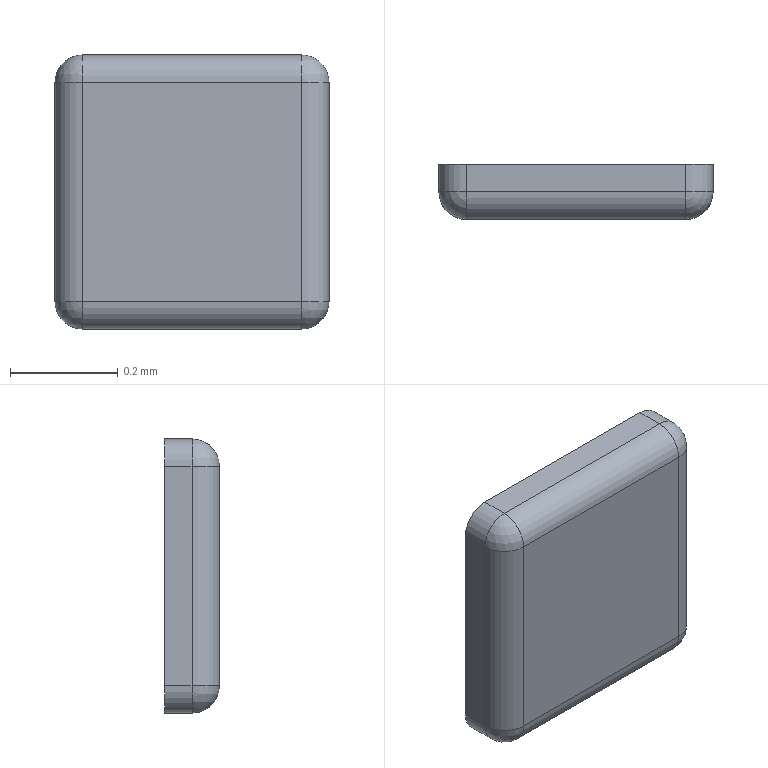Part | STEP file | RJ-USIO-V1_2-220411_2 | 1 solid | 18 faces | box 0.508 x 0.1016 x 0.508 mm | volume 0.02496 mm3 | cylinder 8 | plane 6 | sphere 4 | commonest cylinder face diameters 0.102 x8
STEP:
#1=CARTESIAN_POINT('',(0.,0.,0.));
#2=DIRECTION('',(0.,0.,1.));
#3=DIRECTION('',(1.,0.,0.));
#4=AXIS2_PLACEMENT_3D('',#1,#2,#3);
#5=CARTESIAN_POINT('',(66.597,38.294,0.000000009));
#6=VERTEX_POINT('',#5);
#7=CARTESIAN_POINT('',(67.003,38.294,-0.000000009));
#8=VERTEX_POINT('',#7);
#9=CARTESIAN_POINT('',(66.597,38.294,0.000000009));
#10=DIRECTION('',(1.,0.000000044,-0.000000044));
#11=VECTOR('',#10,1.);
#12=LINE('',#9,#11);
#13=CARTESIAN_POINT('',(67.054,38.294,0.508));
#14=DIRECTION('',(-0.000000044,1.,0.));
#15=DIRECTION('',(1.,0.000000044,-0.000000044));
#16=AXIS2_PLACEMENT_3D('',#13,#14,#15);
#17=PLANE('',#16);
#18=CARTESIAN_POINT('',(-0.4572,0.508));
#19=DIRECTION('',(1.,0.));
#20=VECTOR('',#19,1.);
#21=LINE('',#18,#20);
#22=(GEOMETRIC_REPRESENTATION_CONTEXT(2)PARAMETRIC_REPRESENTATION_CONTEXT()REPRESENTATION_CONTEXT('',''));
#23=DEFINITIONAL_REPRESENTATION('',(#21),#22);
#24=PCURVE('',#17,#23);
#25=CARTESIAN_POINT('',(66.546,38.192,0.000000011));
#26=DIRECTION('',(0.000000044,0.,1.));
#27=DIRECTION('',(-1.,-0.000000044,0.000000044));
#28=AXIS2_PLACEMENT_3D('',#25,#26,#27);
#29=PLANE('',#28);
#30=CARTESIAN_POINT('',(-0.0508,-0.1016));
#31=DIRECTION('',(-1.,0.));
#32=VECTOR('',#31,1.);
#33=LINE('',#30,#32);
#34=(GEOMETRIC_REPRESENTATION_CONTEXT(2)PARAMETRIC_REPRESENTATION_CONTEXT()REPRESENTATION_CONTEXT('',''));
#35=DEFINITIONAL_REPRESENTATION('',(#33),#34);
#36=PCURVE('',#29,#35);
#37=SURFACE_CURVE('',#12,(#24,#36),.PCURVE_S1.);
#38=EDGE_CURVE('',#6,#8,#37,.T.);
#39=ORIENTED_EDGE('',*,*,#38,.T.);
#40=CARTESIAN_POINT('',(67.054,38.294,0.0508));
#41=VERTEX_POINT('',#40);
#42=CARTESIAN_POINT('',(67.003,38.294,0.0508));
#43=DIRECTION('',(-0.000000044,1.,0.));
#44=DIRECTION('',(1.,0.000000044,-0.000000044));
#45=AXIS2_PLACEMENT_3D('',#42,#43,#44);
#46=CIRCLE('',#45,0.0508);
#47=CARTESIAN_POINT('',(-0.0508,0.4572));
#48=DIRECTION('',(1.,0.));
#49=AXIS2_PLACEMENT_2D('',#47,#48);
#50=CIRCLE('',#49,0.0508);
#51=(GEOMETRIC_REPRESENTATION_CONTEXT(2)PARAMETRIC_REPRESENTATION_CONTEXT()REPRESENTATION_CONTEXT('',''));
#52=DEFINITIONAL_REPRESENTATION('',(#50),#51);
#53=PCURVE('',#17,#52);
#54=CARTESIAN_POINT('',(67.003,38.192,0.0508));
#55=DIRECTION('',(-0.000000044,1.,0.));
#56=DIRECTION('',(1.,0.000000044,-0.000000044));
#57=AXIS2_PLACEMENT_3D('',#54,#55,#56);
#58=CYLINDRICAL_SURFACE('',#57,0.0508);
#59=CARTESIAN_POINT('',(0.,0.1016));
#60=DIRECTION('',(1.,0.));
#61=VECTOR('',#60,1.);
#62=LINE('',#59,#61);
#63=(GEOMETRIC_REPRESENTATION_CONTEXT(2)PARAMETRIC_REPRESENTATION_CONTEXT()REPRESENTATION_CONTEXT('',''));
#64=DEFINITIONAL_REPRESENTATION('',(#62),#63);
#65=PCURVE('',#58,#64);
#66=SURFACE_CURVE('',#46,(#53,#65),.PCURVE_S1.);
#67=EDGE_CURVE('',#41,#8,#66,.T.);
#68=ORIENTED_EDGE('',*,*,#67,.F.);
#69=CARTESIAN_POINT('',(67.054,38.294,0.4572));
#70=VERTEX_POINT('',#69);
#71=CARTESIAN_POINT('',(67.054,38.294,0.0508));
#72=DIRECTION('',(0.000000044,0.,1.));
#73=VECTOR('',#72,1.);
#74=LINE('',#71,#73);
#75=CARTESIAN_POINT('',(0.,0.4572));
#76=DIRECTION('',(0.,-1.));
#77=VECTOR('',#76,1.);
#78=LINE('',#75,#77);
#79=(GEOMETRIC_REPRESENTATION_CONTEXT(2)PARAMETRIC_REPRESENTATION_CONTEXT()REPRESENTATION_CONTEXT('',''));
#80=DEFINITIONAL_REPRESENTATION('',(#78),#79);
#81=PCURVE('',#17,#80);
#82=CARTESIAN_POINT('',(67.054,38.192,-0.000000011));
#83=DIRECTION('',(-1.,-0.000000044,0.000000044));
#84=DIRECTION('',(-0.000000044,1.,0.));
#85=AXIS2_PLACEMENT_3D('',#82,#83,#84);
#86=PLANE('',#85);
#87=CARTESIAN_POINT('',(0.1016,-0.0508));
#88=DIRECTION('',(0.,-1.));
#89=VECTOR('',#88,1.);
#90=LINE('',#87,#89);
#91=(GEOMETRIC_REPRESENTATION_CONTEXT(2)PARAMETRIC_REPRESENTATION_CONTEXT()REPRESENTATION_CONTEXT('',''));
#92=DEFINITIONAL_REPRESENTATION('',(#90),#91);
#93=PCURVE('',#86,#92);
#94=SURFACE_CURVE('',#74,(#81,#93),.PCURVE_S1.);
#95=EDGE_CURVE('',#41,#70,#94,.T.);
#96=ORIENTED_EDGE('',*,*,#95,.T.);
#97=CARTESIAN_POINT('',(67.003,38.294,0.508));
#98=VERTEX_POINT('',#97);
#99=CARTESIAN_POINT('',(67.003,38.294,0.4572));
#100=DIRECTION('',(-0.000000044,1.,0.));
#101=DIRECTION('',(0.000000044,0.,1.));
#102=AXIS2_PLACEMENT_3D('',#99,#100,#101);
#103=CIRCLE('',#102,0.0508);
#104=CARTESIAN_POINT('',(-0.0508,0.0508));
#105=DIRECTION('',(0.,-1.));
#106=AXIS2_PLACEMENT_2D('',#104,#105);
#107=CIRCLE('',#106,0.0508);
#108=(GEOMETRIC_REPRESENTATION_CONTEXT(2)PARAMETRIC_REPRESENTATION_CONTEXT()REPRESENTATION_CONTEXT('',''));
#109=DEFINITIONAL_REPRESENTATION('',(#107),#108);
#110=PCURVE('',#17,#109);
#111=CARTESIAN_POINT('',(67.003,38.192,0.4572));
#112=DIRECTION('',(-0.000000044,1.,0.));
#113=DIRECTION('',(1.,0.000000044,-0.000000044));
#114=AXIS2_PLACEMENT_3D('',#111,#112,#113);
#115=CYLINDRICAL_SURFACE('',#114,0.0508);
#116=CARTESIAN_POINT('',(4.712,0.1016));
#117=DIRECTION('',(1.,0.));
#118=VECTOR('',#117,1.);
#119=LINE('',#116,#118);
#120=(GEOMETRIC_REPRESENTATION_CONTEXT(2)PARAMETRIC_REPRESENTATION_CONTEXT()REPRESENTATION_CONTEXT('',''));
#121=DEFINITIONAL_REPRESENTATION('',(#119),#120);
#122=PCURVE('',#115,#121);
#123=SURFACE_CURVE('',#103,(#110,#122),.PCURVE_S1.);
#124=EDGE_CURVE('',#98,#70,#123,.T.);
#125=ORIENTED_EDGE('',*,*,#124,.F.);
#126=CARTESIAN_POINT('',(66.597,38.294,0.508));
#127=VERTEX_POINT('',#126);
#128=CARTESIAN_POINT('',(67.003,38.294,0.508));
#129=DIRECTION('',(-1.,-0.000000044,0.000000044));
#130=VECTOR('',#129,1.);
#131=LINE('',#128,#130);
#132=CARTESIAN_POINT('',(-0.0508,0.));
#133=DIRECTION('',(-1.,0.));
#134=VECTOR('',#133,1.);
#135=LINE('',#132,#134);
#136=(GEOMETRIC_REPRESENTATION_CONTEXT(2)PARAMETRIC_REPRESENTATION_CONTEXT()REPRESENTATION_CONTEXT('',''));
#137=DEFINITIONAL_REPRESENTATION('',(#135),#136);
#138=PCURVE('',#17,#137);
#139=CARTESIAN_POINT('',(66.546,38.192,0.508));
#140=DIRECTION('',(-0.000000044,0.,-1.));
#141=DIRECTION('',(1.,0.000000044,-0.000000044));
#142=AXIS2_PLACEMENT_3D('',#139,#140,#141);
#143=PLANE('',#142);
#144=CARTESIAN_POINT('',(0.4572,-0.1016));
#145=DIRECTION('',(-1.,0.));
#146=VECTOR('',#145,1.);
#147=LINE('',#144,#146);
#148=(GEOMETRIC_REPRESENTATION_CONTEXT(2)PARAMETRIC_REPRESENTATION_CONTEXT()REPRESENTATION_CONTEXT('',''));
#149=DEFINITIONAL_REPRESENTATION('',(#147),#148);
#150=PCURVE('',#143,#149);
#151=SURFACE_CURVE('',#131,(#138,#150),.PCURVE_S1.);
#152=EDGE_CURVE('',#98,#127,#151,.T.);
#153=ORIENTED_EDGE('',*,*,#152,.T.);
#154=CARTESIAN_POINT('',(66.546,38.294,0.4572));
#155=VERTEX_POINT('',#154);
#156=CARTESIAN_POINT('',(66.597,38.294,0.4572));
#157=DIRECTION('',(-0.000000044,1.,0.));
#158=DIRECTION('',(-1.,-0.000000044,0.000000044));
#159=AXIS2_PLACEMENT_3D('',#156,#157,#158);
#160=CIRCLE('',#159,0.0508);
#161=CARTESIAN_POINT('',(-0.4572,0.0508));
#162=DIRECTION('',(-1.,0.));
#163=AXIS2_PLACEMENT_2D('',#161,#162);
#164=CIRCLE('',#163,0.0508);
#165=(GEOMETRIC_REPRESENTATION_CONTEXT(2)PARAMETRIC_REPRESENTATION_CONTEXT()REPRESENTATION_CONTEXT('',''));
#166=DEFINITIONAL_REPRESENTATION('',(#164),#165);
#167=PCURVE('',#17,#166);
#168=CARTESIAN_POINT('',(66.597,38.192,0.4572));
#169=DIRECTION('',(-0.000000044,1.,0.));
#170=DIRECTION('',(1.,0.000000044,-0.000000044));
#171=AXIS2_PLACEMENT_3D('',#168,#169,#170);
#172=CYLINDRICAL_SURFACE('',#171,0.0508);
#173=CARTESIAN_POINT('',(3.142,0.1016));
#174=DIRECTION('',(1.,0.));
#175=VECTOR('',#174,1.);
#176=LINE('',#173,#175);
#177=(GEOMETRIC_REPRESENTATION_CONTEXT(2)PARAMETRIC_REPRESENTATION_CONTEXT()REPRESENTATION_CONTEXT('',''));
#178=DEFINITIONAL_REPRESENTATION('',(#176),#177);
#179=PCURVE('',#172,#178);
#180=SURFACE_CURVE('',#160,(#167,#179),.PCURVE_S1.);
#181=EDGE_CURVE('',#155,#127,#180,.T.);
#182=ORIENTED_EDGE('',*,*,#181,.F.);
#183=CARTESIAN_POINT('',(66.546,38.294,0.0508));
#184=VERTEX_POINT('',#183);
#185=CARTESIAN_POINT('',(66.546,38.294,0.4572));
#186=DIRECTION('',(-0.000000044,0.,-1.));
#187=VECTOR('',#186,1.);
#188=LINE('',#185,#187);
#189=CARTESIAN_POINT('',(-0.508,0.0508));
#190=DIRECTION('',(0.,1.));
#191=VECTOR('',#190,1.);
#192=LINE('',#189,#191);
#193=(GEOMETRIC_REPRESENTATION_CONTEXT(2)PARAMETRIC_REPRESENTATION_CONTEXT()REPRESENTATION_CONTEXT('',''));
#194=DEFINITIONAL_REPRESENTATION('',(#192),#193);
#195=PCURVE('',#17,#194);
#196=CARTESIAN_POINT('',(66.546,38.192,0.000000011));
#197=DIRECTION('',(1.,0.000000044,-0.000000044));
#198=DIRECTION('',(0.000000044,-1.,0.));
#199=AXIS2_PLACEMENT_3D('',#196,#197,#198);
#200=PLANE('',#199);
#201=CARTESIAN_POINT('',(-0.1016,-0.4572));
#202=DIRECTION('',(0.,1.));
#203=VECTOR('',#202,1.);
#204=LINE('',#201,#203);
#205=(GEOMETRIC_REPRESENTATION_CONTEXT(2)PARAMETRIC_REPRESENTATION_CONTEXT()REPRESENTATION_CONTEXT('',''));
#206=DEFINITIONAL_REPRESENTATION('',(#204),#205);
#207=PCURVE('',#200,#206);
#208=SURFACE_CURVE('',#188,(#195,#207),.PCURVE_S1.);
#209=EDGE_CURVE('',#155,#184,#208,.T.);
#210=ORIENTED_EDGE('',*,*,#209,.T.);
#211=CARTESIAN_POINT('',(66.597,38.294,0.0508));
#212=DIRECTION('',(-0.000000044,1.,0.));
#213=DIRECTION('',(-0.000000044,0.,-1.));
#214=AXIS2_PLACEMENT_3D('',#211,#212,#213);
#215=CIRCLE('',#214,0.0508);
#216=CARTESIAN_POINT('',(-0.4572,0.4572));
#217=DIRECTION('',(0.,1.));
#218=AXIS2_PLACEMENT_2D('',#216,#217);
#219=CIRCLE('',#218,0.0508);
#220=(GEOMETRIC_REPRESENTATION_CONTEXT(2)PARAMETRIC_REPRESENTATION_CONTEXT()REPRESENTATION_CONTEXT('',''));
#221=DEFINITIONAL_REPRESENTATION('',(#219),#220);
#222=PCURVE('',#17,#221);
#223=CARTESIAN_POINT('',(66.597,38.192,0.0508));
#224=DIRECTION('',(-0.000000044,1.,0.));
#225=DIRECTION('',(1.,0.000000044,-0.000000044));
#226=AXIS2_PLACEMENT_3D('',#223,#224,#225);
#227=CYLINDRICAL_SURFACE('',#226,0.0508);
#228=CARTESIAN_POINT('',(1.571,0.1016));
#229=DIRECTION('',(1.,0.));
#230=VECTOR('',#229,1.);
#231=LINE('',#228,#230);
#232=(GEOMETRIC_REPRESENTATION_CONTEXT(2)PARAMETRIC_REPRESENTATION_CONTEXT()REPRESENTATION_CONTEXT('',''));
#233=DEFINITIONAL_REPRESENTATION('',(#231),#232);
#234=PCURVE('',#227,#233);
#235=SURFACE_CURVE('',#215,(#222,#234),.PCURVE_S1.);
#236=EDGE_CURVE('',#6,#184,#235,.T.);
#237=ORIENTED_EDGE('',*,*,#236,.F.);
#238=EDGE_LOOP('',(#39,#68,#96,#125,#153,#182,#210,#237));
#239=FACE_BOUND('',#238,.F.);
#240=ADVANCED_FACE('',(#239),#17,.T.);
#241=CARTESIAN_POINT('',(66.597,38.243,0.000000009));
#242=VERTEX_POINT('',#241);
#243=CARTESIAN_POINT('',(67.003,38.243,-0.000000009));
#244=VERTEX_POINT('',#243);
#245=CARTESIAN_POINT('',(66.597,38.243,0.000000009));
#246=DIRECTION('',(1.,0.000000044,-0.000000044));
#247=VECTOR('',#246,1.);
#248=LINE('',#245,#247);
#249=CARTESIAN_POINT('',(-0.0508,-0.0508));
#250=DIRECTION('',(-1.,0.));
#251=VECTOR('',#250,1.);
#252=LINE('',#249,#251);
#253=(GEOMETRIC_REPRESENTATION_CONTEXT(2)PARAMETRIC_REPRESENTATION_CONTEXT()REPRESENTATION_CONTEXT('',''));
#254=DEFINITIONAL_REPRESENTATION('',(#252),#253);
#255=PCURVE('',#29,#254);
#256=CARTESIAN_POINT('',(67.054,38.243,0.0508));
#257=DIRECTION('',(1.,0.000000044,-0.000000044));
#258=DIRECTION('',(0.000000044,-1.,0.));
#259=AXIS2_PLACEMENT_3D('',#256,#257,#258);
#260=CYLINDRICAL_SURFACE('',#259,0.0508);
#261=CARTESIAN_POINT('',(1.571,-0.4572));
#262=DIRECTION('',(0.,1.));
#263=VECTOR('',#262,1.);
#264=LINE('',#261,#263);
#265=(GEOMETRIC_REPRESENTATION_CONTEXT(2)PARAMETRIC_REPRESENTATION_CONTEXT()REPRESENTATION_CONTEXT('',''));
#266=DEFINITIONAL_REPRESENTATION('',(#264),#265);
#267=PCURVE('',#260,#266);
#268=SURFACE_CURVE('',#248,(#255,#267),.PCURVE_S1.);
#269=EDGE_CURVE('',#242,#244,#268,.T.);
#270=ORIENTED_EDGE('',*,*,#269,.T.);
#271=CARTESIAN_POINT('',(67.003,38.243,-0.000000009));
#272=DIRECTION('',(-0.000000044,1.,0.));
#273=VECTOR('',#272,1.);
#274=LINE('',#271,#273);
#275=CARTESIAN_POINT('',(-0.4572,-0.0508));
#276=DIRECTION('',(0.,-1.));
#277=VECTOR('',#276,1.);
#278=LINE('',#275,#277);
#279=(GEOMETRIC_REPRESENTATION_CONTEXT(2)PARAMETRIC_REPRESENTATION_CONTEXT()REPRESENTATION_CONTEXT('',''));
#280=DEFINITIONAL_REPRESENTATION('',(#278),#279);
#281=PCURVE('',#29,#280);
#282=CARTESIAN_POINT('',(1.571,0.0508));
#283=DIRECTION('',(0.,1.));
#284=VECTOR('',#283,1.);
#285=LINE('',#282,#284);
#286=(GEOMETRIC_REPRESENTATION_CONTEXT(2)PARAMETRIC_REPRESENTATION_CONTEXT()REPRESENTATION_CONTEXT('',''));
#287=DEFINITIONAL_REPRESENTATION('',(#285),#286);
#288=PCURVE('',#58,#287);
#289=SURFACE_CURVE('',#274,(#281,#288),.PCURVE_S1.);
#290=EDGE_CURVE('',#244,#8,#289,.T.);
#291=ORIENTED_EDGE('',*,*,#290,.T.);
#292=ORIENTED_EDGE('',*,*,#38,.F.);
#293=CARTESIAN_POINT('',(66.597,38.294,0.000000009));
#294=DIRECTION('',(0.000000044,-1.,0.));
#295=VECTOR('',#294,1.);
#296=LINE('',#293,#295);
#297=CARTESIAN_POINT('',(-0.0508,-0.1016));
#298=DIRECTION('',(0.,1.));
#299=VECTOR('',#298,1.);
#300=LINE('',#297,#299);
#301=(GEOMETRIC_REPRESENTATION_CONTEXT(2)PARAMETRIC_REPRESENTATION_CONTEXT()REPRESENTATION_CONTEXT('',''));
#302=DEFINITIONAL_REPRESENTATION('',(#300),#301);
#303=PCURVE('',#29,#302);
#304=CARTESIAN_POINT('',(1.571,0.1016));
#305=DIRECTION('',(0.,-1.));
#306=VECTOR('',#305,1.);
#307=LINE('',#304,#306);
#308=(GEOMETRIC_REPRESENTATION_CONTEXT(2)PARAMETRIC_REPRESENTATION_CONTEXT()REPRESENTATION_CONTEXT('',''));
#309=DEFINITIONAL_REPRESENTATION('',(#307),#308);
#310=PCURVE('',#227,#309);
#311=SURFACE_CURVE('',#296,(#303,#310),.PCURVE_S1.);
#312=EDGE_CURVE('',#6,#242,#311,.T.);
#313=ORIENTED_EDGE('',*,*,#312,.T.);
#314=EDGE_LOOP('',(#270,#291,#292,#313));
#315=FACE_BOUND('',#314,.F.);
#316=ADVANCED_FACE('',(#315),#29,.F.);
#317=CARTESIAN_POINT('',(67.003,38.192,0.0508));
#318=VERTEX_POINT('',#317);
#319=CARTESIAN_POINT('',(66.597,38.192,0.0508));
#320=VERTEX_POINT('',#319);
#321=CARTESIAN_POINT('',(67.003,38.192,0.0508));
#322=DIRECTION('',(-1.,-0.000000044,0.000000044));
#323=VECTOR('',#322,1.);
#324=LINE('',#321,#323);
#325=CARTESIAN_POINT('',(0.,-0.0508));
#326=DIRECTION('',(0.,-1.));
#327=VECTOR('',#326,1.);
#328=LINE('',#325,#327);
#329=(GEOMETRIC_REPRESENTATION_CONTEXT(2)PARAMETRIC_REPRESENTATION_CONTEXT()REPRESENTATION_CONTEXT('',''));
#330=DEFINITIONAL_REPRESENTATION('',(#328),#329);
#331=PCURVE('',#260,#330);
#332=CARTESIAN_POINT('',(67.054,38.192,0.508));
#333=DIRECTION('',(-0.000000044,1.,0.));
#334=DIRECTION('',(1.,0.000000044,-0.000000044));
#335=AXIS2_PLACEMENT_3D('',#332,#333,#334);
#336=PLANE('',#335);
#337=CARTESIAN_POINT('',(-0.0508,0.4572));
#338=DIRECTION('',(-1.,0.));
#339=VECTOR('',#338,1.);
#340=LINE('',#337,#339);
#341=(GEOMETRIC_REPRESENTATION_CONTEXT(2)PARAMETRIC_REPRESENTATION_CONTEXT()REPRESENTATION_CONTEXT('',''));
#342=DEFINITIONAL_REPRESENTATION('',(#340),#341);
#343=PCURVE('',#336,#342);
#344=SURFACE_CURVE('',#324,(#331,#343),.PCURVE_S1.);
#345=EDGE_CURVE('',#318,#320,#344,.T.);
#346=ORIENTED_EDGE('',*,*,#345,.T.);
#347=CARTESIAN_POINT('',(66.597,38.243,0.0508));
#348=DIRECTION('',(-1.,-0.000000044,0.000000044));
#349=DIRECTION('',(-0.000000044,0.,-1.));
#350=AXIS2_PLACEMENT_3D('',#347,#348,#349);
#351=CIRCLE('',#350,0.0508);
#352=CARTESIAN_POINT('',(1.571,-0.4572));
#353=DIRECTION('',(-1.,0.));
#354=VECTOR('',#353,1.);
#355=LINE('',#352,#354);
#356=(GEOMETRIC_REPRESENTATION_CONTEXT(2)PARAMETRIC_REPRESENTATION_CONTEXT()REPRESENTATION_CONTEXT('',''));
#357=DEFINITIONAL_REPRESENTATION('',(#355),#356);
#358=PCURVE('',#260,#357);
#359=CARTESIAN_POINT('',(66.597,38.243,0.0508));
#360=DIRECTION('',(0.000000044,0.,1.));
#361=DIRECTION('',(1.,0.000000044,-0.000000044));
#362=AXIS2_PLACEMENT_3D('',#359,#360,#361);
#363=SPHERICAL_SURFACE('',#362,0.0508);
#364=CARTESIAN_POINT('',(4.712,-1.571));
#365=DIRECTION('',(0.,1.));
#366=VECTOR('',#365,1.);
#367=LINE('',#364,#366);
#368=(GEOMETRIC_REPRESENTATION_CONTEXT(2)PARAMETRIC_REPRESENTATION_CONTEXT()REPRESENTATION_CONTEXT('',''));
#369=DEFINITIONAL_REPRESENTATION('',(#367),#368);
#370=PCURVE('',#363,#369);
#371=SURFACE_CURVE('',#351,(#358,#370),.PCURVE_S1.);
#372=EDGE_CURVE('',#242,#320,#371,.T.);
#373=ORIENTED_EDGE('',*,*,#372,.F.);
#374=ORIENTED_EDGE('',*,*,#269,.T.);
#375=CARTESIAN_POINT('',(67.003,38.243,0.0508));
#376=DIRECTION('',(1.,0.000000044,-0.000000044));
#377=DIRECTION('',(0.000000044,-1.,0.));
#378=AXIS2_PLACEMENT_3D('',#375,#376,#377);
#379=CIRCLE('',#378,0.0508);
#380=CARTESIAN_POINT('',(0.,-0.0508));
#381=DIRECTION('',(1.,0.));
#382=VECTOR('',#381,1.);
#383=LINE('',#380,#382);
#384=(GEOMETRIC_REPRESENTATION_CONTEXT(2)PARAMETRIC_REPRESENTATION_CONTEXT()REPRESENTATION_CONTEXT('',''));
#385=DEFINITIONAL_REPRESENTATION('',(#383),#384);
#386=PCURVE('',#260,#385);
#387=CARTESIAN_POINT('',(67.003,38.243,0.0508));
#388=DIRECTION('',(0.000000044,0.,1.));
#389=DIRECTION('',(1.,0.000000044,-0.000000044));
#390=AXIS2_PLACEMENT_3D('',#387,#388,#389);
#391=SPHERICAL_SURFACE('',#390,0.0508);
#392=CARTESIAN_POINT('',(4.712,0.));
#393=CARTESIAN_POINT('',(4.712,-0.0238));
#394=CARTESIAN_POINT('',(4.712,-0.0714));
#395=CARTESIAN_POINT('',(4.712,-0.1428));
#396=CARTESIAN_POINT('',(4.712,-0.2142));
#397=CARTESIAN_POINT('',(4.712,-0.2856));
#398=CARTESIAN_POINT('',(4.712,-0.357));
#399=CARTESIAN_POINT('',(4.712,-0.4284));
#400=CARTESIAN_POINT('',(4.712,-0.4998));
#401=CARTESIAN_POINT('',(4.712,-0.5712));
#402=CARTESIAN_POINT('',(4.712,-0.6426));
#403=CARTESIAN_POINT('',(4.712,-0.714));
#404=CARTESIAN_POINT('',(4.712,-0.7854));
#405=CARTESIAN_POINT('',(4.712,-0.8568));
#406=CARTESIAN_POINT('',(4.712,-0.9282));
#407=CARTESIAN_POINT('',(4.712,-0.9996));
#408=CARTESIAN_POINT('',(4.712,-1.071));
#409=CARTESIAN_POINT('',(4.712,-1.142));
#410=CARTESIAN_POINT('',(4.712,-1.214));
#411=CARTESIAN_POINT('',(4.712,-1.285));
#412=CARTESIAN_POINT('',(4.712,-1.357));
#413=CARTESIAN_POINT('',(4.712,-1.428));
#414=CARTESIAN_POINT('',(4.712,-1.499));
#415=CARTESIAN_POINT('',(4.712,-1.547));
#416=CARTESIAN_POINT('',(4.712,-1.571));
#417=B_SPLINE_CURVE_WITH_KNOTS('',3,(#392,#393,#394,#395,#396,#397,#398,#399,#400,#401,#402,#403,#404,#405,#406,#407,#408,#409,#410,#411,#412,#413,#414,#415,#416),.UNSPECIFIED.,.F.,.F.,(4,1,1,1,1,1,1,1,1,1,1,1,1,1,1,1,1,1,1,1,1,1,4),(0.,0.0714,0.1428,0.2142,0.2856,0.357,0.4284,0.4998,0.5712,0.6426,0.714,0.7854,0.8568,0.9282,0.9996,1.071,1.142,1.214,1.285,1.357,1.428,1.499,1.571),.QUASI_UNIFORM_KNOTS.);
#418=(GEOMETRIC_REPRESENTATION_CONTEXT(2)PARAMETRIC_REPRESENTATION_CONTEXT()REPRESENTATION_CONTEXT('',''));
#419=DEFINITIONAL_REPRESENTATION('',(#417),#418);
#420=PCURVE('',#391,#419);
#421=SURFACE_CURVE('',#379,(#386,#420),.PCURVE_S1.);
#422=EDGE_CURVE('',#318,#244,#421,.T.);
#423=ORIENTED_EDGE('',*,*,#422,.F.);
#424=EDGE_LOOP('',(#346,#373,#374,#423));
#425=FACE_BOUND('',#424,.T.);
#426=ADVANCED_FACE('',(#425),#260,.T.);
#427=CARTESIAN_POINT('',(67.054,38.243,0.0508));
#428=VERTEX_POINT('',#427);
#429=CARTESIAN_POINT('',(67.003,38.243,0.0508));
#430=DIRECTION('',(-0.000000044,0.,-1.));
#431=DIRECTION('',(1.,0.000000044,-0.000000044));
#432=AXIS2_PLACEMENT_3D('',#429,#430,#431);
#433=CIRCLE('',#432,0.0508);
#434=CARTESIAN_POINT('',(6.283,0.));
#435=DIRECTION('',(-1.,0.));
#436=VECTOR('',#435,1.);
#437=LINE('',#434,#436);
#438=(GEOMETRIC_REPRESENTATION_CONTEXT(2)PARAMETRIC_REPRESENTATION_CONTEXT()REPRESENTATION_CONTEXT('',''));
#439=DEFINITIONAL_REPRESENTATION('',(#437),#438);
#440=PCURVE('',#391,#439);
#441=CARTESIAN_POINT('',(67.003,38.243,0.508));
#442=DIRECTION('',(0.000000044,0.,1.));
#443=DIRECTION('',(-1.,-0.000000044,0.000000044));
#444=AXIS2_PLACEMENT_3D('',#441,#442,#443);
#445=CYLINDRICAL_SURFACE('',#444,0.0508);
#446=CARTESIAN_POINT('',(3.142,-0.4572));
#447=DIRECTION('',(-1.,0.));
#448=VECTOR('',#447,1.);
#449=LINE('',#446,#448);
#450=(GEOMETRIC_REPRESENTATION_CONTEXT(2)PARAMETRIC_REPRESENTATION_CONTEXT()REPRESENTATION_CONTEXT('',''));
#451=DEFINITIONAL_REPRESENTATION('',(#449),#450);
#452=PCURVE('',#445,#451);
#453=SURFACE_CURVE('',#433,(#440,#452),.PCURVE_S1.);
#454=EDGE_CURVE('',#428,#318,#453,.T.);
#455=ORIENTED_EDGE('',*,*,#454,.T.);
#456=ORIENTED_EDGE('',*,*,#422,.T.);
#457=CARTESIAN_POINT('',(67.003,38.243,0.0508));
#458=DIRECTION('',(0.000000044,-1.,0.));
#459=DIRECTION('',(-0.000000044,0.,-1.));
#460=AXIS2_PLACEMENT_3D('',#457,#458,#459);
#461=CIRCLE('',#460,0.0508);
#462=CARTESIAN_POINT('',(6.283,-1.571));
#463=DIRECTION('',(0.,1.));
#464=VECTOR('',#463,1.);
#465=LINE('',#462,#464);
#466=(GEOMETRIC_REPRESENTATION_CONTEXT(2)PARAMETRIC_REPRESENTATION_CONTEXT()REPRESENTATION_CONTEXT('',''));
#467=DEFINITIONAL_REPRESENTATION('',(#465),#466);
#468=PCURVE('',#391,#467);
#469=CARTESIAN_POINT('',(1.571,0.0508));
#470=DIRECTION('',(-1.,0.));
#471=VECTOR('',#470,1.);
#472=LINE('',#469,#471);
#473=(GEOMETRIC_REPRESENTATION_CONTEXT(2)PARAMETRIC_REPRESENTATION_CONTEXT()REPRESENTATION_CONTEXT('',''));
#474=DEFINITIONAL_REPRESENTATION('',(#472),#473);
#475=PCURVE('',#58,#474);
#476=SURFACE_CURVE('',#461,(#468,#475),.PCURVE_S1.);
#477=EDGE_CURVE('',#244,#428,#476,.T.);
#478=ORIENTED_EDGE('',*,*,#477,.T.);
#479=EDGE_LOOP('',(#455,#456,#478));
#480=FACE_BOUND('',#479,.T.);
#481=ADVANCED_FACE('',(#480),#391,.T.);
#482=ORIENTED_EDGE('',*,*,#67,.F.);
#483=CARTESIAN_POINT('',(67.054,38.294,0.0508));
#484=DIRECTION('',(0.000000044,-1.,0.));
#485=VECTOR('',#484,1.);
#486=LINE('',#483,#485);
#487=CARTESIAN_POINT('',(0.,0.1016));
#488=DIRECTION('',(0.,-1.));
#489=VECTOR('',#488,1.);
#490=LINE('',#487,#489);
#491=(GEOMETRIC_REPRESENTATION_CONTEXT(2)PARAMETRIC_REPRESENTATION_CONTEXT()REPRESENTATION_CONTEXT('',''));
#492=DEFINITIONAL_REPRESENTATION('',(#490),#491);
#493=PCURVE('',#58,#492);
#494=CARTESIAN_POINT('',(0.1016,-0.0508));
#495=DIRECTION('',(-1.,0.));
#496=VECTOR('',#495,1.);
#497=LINE('',#494,#496);
#498=(GEOMETRIC_REPRESENTATION_CONTEXT(2)PARAMETRIC_REPRESENTATION_CONTEXT()REPRESENTATION_CONTEXT('',''));
#499=DEFINITIONAL_REPRESENTATION('',(#497),#498);
#500=PCURVE('',#86,#499);
#501=SURFACE_CURVE('',#486,(#493,#500),.PCURVE_S1.);
#502=EDGE_CURVE('',#41,#428,#501,.T.);
#503=ORIENTED_EDGE('',*,*,#502,.T.);
#504=ORIENTED_EDGE('',*,*,#477,.F.);
#505=ORIENTED_EDGE('',*,*,#290,.T.);
#506=EDGE_LOOP('',(#482,#503,#504,#505));
#507=FACE_BOUND('',#506,.T.);
#508=ADVANCED_FACE('',(#507),#58,.T.);
#509=CARTESIAN_POINT('',(67.054,38.243,0.4572));
#510=VERTEX_POINT('',#509);
#511=CARTESIAN_POINT('',(67.054,38.243,0.0508));
#512=DIRECTION('',(0.000000044,0.,1.));
#513=VECTOR('',#512,1.);
#514=LINE('',#511,#513);
#515=CARTESIAN_POINT('',(0.0508,-0.0508));
#516=DIRECTION('',(0.,-1.));
#517=VECTOR('',#516,1.);
#518=LINE('',#515,#517);
#519=(GEOMETRIC_REPRESENTATION_CONTEXT(2)PARAMETRIC_REPRESENTATION_CONTEXT()REPRESENTATION_CONTEXT('',''));
#520=DEFINITIONAL_REPRESENTATION('',(#518),#519);
#521=PCURVE('',#86,#520);
#522=CARTESIAN_POINT('',(3.142,-0.4572));
#523=DIRECTION('',(0.,1.));
#524=VECTOR('',#523,1.);
#525=LINE('',#522,#524);
#526=(GEOMETRIC_REPRESENTATION_CONTEXT(2)PARAMETRIC_REPRESENTATION_CONTEXT()REPRESENTATION_CONTEXT('',''));
#527=DEFINITIONAL_REPRESENTATION('',(#525),#526);
#528=PCURVE('',#445,#527);
#529=SURFACE_CURVE('',#514,(#521,#528),.PCURVE_S1.);
#530=EDGE_CURVE('',#428,#510,#529,.T.);
#531=ORIENTED_EDGE('',*,*,#530,.T.);
#532=CARTESIAN_POINT('',(67.054,38.243,0.4572));
#533=DIRECTION('',(-0.000000044,1.,0.));
#534=VECTOR('',#533,1.);
#535=LINE('',#532,#534);
#536=CARTESIAN_POINT('',(0.0508,-0.4572));
#537=DIRECTION('',(1.,0.));
#538=VECTOR('',#537,1.);
#539=LINE('',#536,#538);
#540=(GEOMETRIC_REPRESENTATION_CONTEXT(2)PARAMETRIC_REPRESENTATION_CONTEXT()REPRESENTATION_CONTEXT('',''));
#541=DEFINITIONAL_REPRESENTATION('',(#539),#540);
#542=PCURVE('',#86,#541);
#543=CARTESIAN_POINT('',(6.283,0.0508));
#544=DIRECTION('',(0.,1.));
#545=VECTOR('',#544,1.);
#546=LINE('',#543,#545);
#547=(GEOMETRIC_REPRESENTATION_CONTEXT(2)PARAMETRIC_REPRESENTATION_CONTEXT()REPRESENTATION_CONTEXT('',''));
#548=DEFINITIONAL_REPRESENTATION('',(#546),#547);
#549=PCURVE('',#115,#548);
#550=SURFACE_CURVE('',#535,(#542,#549),.PCURVE_S1.);
#551=EDGE_CURVE('',#510,#70,#550,.T.);
#552=ORIENTED_EDGE('',*,*,#551,.T.);
#553=ORIENTED_EDGE('',*,*,#95,.F.);
#554=ORIENTED_EDGE('',*,*,#502,.T.);
#555=EDGE_LOOP('',(#531,#552,#553,#554));
#556=FACE_BOUND('',#555,.F.);
#557=ADVANCED_FACE('',(#556),#86,.F.);
#558=CARTESIAN_POINT('',(67.003,38.192,0.4572));
#559=VERTEX_POINT('',#558);
#560=CARTESIAN_POINT('',(67.003,38.192,0.4572));
#561=DIRECTION('',(-0.000000044,0.,-1.));
#562=VECTOR('',#561,1.);
#563=LINE('',#560,#562);
#564=CARTESIAN_POINT('',(1.571,-0.0508));
#565=DIRECTION('',(0.,-1.));
#566=VECTOR('',#565,1.);
#567=LINE('',#564,#566);
#568=(GEOMETRIC_REPRESENTATION_CONTEXT(2)PARAMETRIC_REPRESENTATION_CONTEXT()REPRESENTATION_CONTEXT('',''));
#569=DEFINITIONAL_REPRESENTATION('',(#567),#568);
#570=PCURVE('',#445,#569);
#571=CARTESIAN_POINT('',(-0.0508,0.0508));
#572=DIRECTION('',(0.,1.));
#573=VECTOR('',#572,1.);
#574=LINE('',#571,#573);
#575=(GEOMETRIC_REPRESENTATION_CONTEXT(2)PARAMETRIC_REPRESENTATION_CONTEXT()REPRESENTATION_CONTEXT('',''));
#576=DEFINITIONAL_REPRESENTATION('',(#574),#575);
#577=PCURVE('',#336,#576);
#578=SURFACE_CURVE('',#563,(#570,#577),.PCURVE_S1.);
#579=EDGE_CURVE('',#559,#318,#578,.T.);
#580=ORIENTED_EDGE('',*,*,#579,.T.);
#581=ORIENTED_EDGE('',*,*,#454,.F.);
#582=ORIENTED_EDGE('',*,*,#530,.T.);
#583=CARTESIAN_POINT('',(67.003,38.243,0.4572));
#584=DIRECTION('',(0.000000044,0.,1.));
#585=DIRECTION('',(0.000000044,-1.,0.));
#586=AXIS2_PLACEMENT_3D('',#583,#584,#585);
#587=CIRCLE('',#586,0.0508);
#588=CARTESIAN_POINT('',(1.571,-0.0508));
#589=DIRECTION('',(1.,0.));
#590=VECTOR('',#589,1.);
#591=LINE('',#588,#590);
#592=(GEOMETRIC_REPRESENTATION_CONTEXT(2)PARAMETRIC_REPRESENTATION_CONTEXT()REPRESENTATION_CONTEXT('',''));
#593=DEFINITIONAL_REPRESENTATION('',(#591),#592);
#594=PCURVE('',#445,#593);
#595=CARTESIAN_POINT('',(67.003,38.243,0.4572));
#596=DIRECTION('',(0.000000044,0.,1.));
#597=DIRECTION('',(1.,0.000000044,-0.000000044));
#598=AXIS2_PLACEMENT_3D('',#595,#596,#597);
#599=SPHERICAL_SURFACE('',#598,0.0508);
#600=CARTESIAN_POINT('',(4.712,0.));
#601=DIRECTION('',(1.,0.));
#602=VECTOR('',#601,1.);
#603=LINE('',#600,#602);
#604=(GEOMETRIC_REPRESENTATION_CONTEXT(2)PARAMETRIC_REPRESENTATION_CONTEXT()REPRESENTATION_CONTEXT('',''));
#605=DEFINITIONAL_REPRESENTATION('',(#603),#604);
#606=PCURVE('',#599,#605);
#607=SURFACE_CURVE('',#587,(#594,#606),.PCURVE_S1.);
#608=EDGE_CURVE('',#559,#510,#607,.T.);
#609=ORIENTED_EDGE('',*,*,#608,.F.);
#610=EDGE_LOOP('',(#580,#581,#582,#609));
#611=FACE_BOUND('',#610,.T.);
#612=ADVANCED_FACE('',(#611),#445,.T.);
#613=CARTESIAN_POINT('',(67.003,38.243,0.508));
#614=VERTEX_POINT('',#613);
#615=CARTESIAN_POINT('',(67.003,38.243,0.4572));
#616=DIRECTION('',(1.,0.000000044,-0.000000044));
#617=DIRECTION('',(0.000000044,0.,1.));
#618=AXIS2_PLACEMENT_3D('',#615,#616,#617);
#619=CIRCLE('',#618,0.0508);
#620=CARTESIAN_POINT('',(4.712,1.571));
#621=DIRECTION('',(0.,-1.));
#622=VECTOR('',#621,1.);
#623=LINE('',#620,#622);
#624=(GEOMETRIC_REPRESENTATION_CONTEXT(2)PARAMETRIC_REPRESENTATION_CONTEXT()REPRESENTATION_CONTEXT('',''));
#625=DEFINITIONAL_REPRESENTATION('',(#623),#624);
#626=PCURVE('',#599,#625);
#627=CARTESIAN_POINT('',(67.054,38.243,0.4572));
#628=DIRECTION('',(-1.,-0.000000044,0.000000044));
#629=DIRECTION('',(-0.000000044,1.,0.));
#630=AXIS2_PLACEMENT_3D('',#627,#628,#629);
#631=CYLINDRICAL_SURFACE('',#630,0.0508);
#632=CARTESIAN_POINT('',(4.712,0.0508));
#633=DIRECTION('',(-1.,0.));
#634=VECTOR('',#633,1.);
#635=LINE('',#632,#634);
#636=(GEOMETRIC_REPRESENTATION_CONTEXT(2)PARAMETRIC_REPRESENTATION_CONTEXT()REPRESENTATION_CONTEXT('',''));
#637=DEFINITIONAL_REPRESENTATION('',(#635),#636);
#638=PCURVE('',#631,#637);
#639=SURFACE_CURVE('',#619,(#626,#638),.PCURVE_S1.);
#640=EDGE_CURVE('',#614,#559,#639,.T.);
#641=ORIENTED_EDGE('',*,*,#640,.T.);
#642=ORIENTED_EDGE('',*,*,#608,.T.);
#643=CARTESIAN_POINT('',(67.003,38.243,0.4572));
#644=DIRECTION('',(0.000000044,-1.,0.));
#645=DIRECTION('',(1.,0.000000044,-0.000000044));
#646=AXIS2_PLACEMENT_3D('',#643,#644,#645);
#647=CIRCLE('',#646,0.0508);
#648=CARTESIAN_POINT('',(6.283,0.));
#649=CARTESIAN_POINT('',(6.283,0.0238));
#650=CARTESIAN_POINT('',(6.283,0.0714));
#651=CARTESIAN_POINT('',(6.283,0.1428));
#652=CARTESIAN_POINT('',(6.283,0.2142));
#653=CARTESIAN_POINT('',(6.283,0.2856));
#654=CARTESIAN_POINT('',(6.283,0.357));
#655=CARTESIAN_POINT('',(6.283,0.4284));
#656=CARTESIAN_POINT('',(6.283,0.4998));
#657=CARTESIAN_POINT('',(6.283,0.5712));
#658=CARTESIAN_POINT('',(6.283,0.6426));
#659=CARTESIAN_POINT('',(6.283,0.714));
#660=CARTESIAN_POINT('',(6.283,0.7854));
#661=CARTESIAN_POINT('',(6.283,0.8568));
#662=CARTESIAN_POINT('',(6.283,0.9282));
#663=CARTESIAN_POINT('',(6.283,0.9996));
#664=CARTESIAN_POINT('',(6.283,1.071));
#665=CARTESIAN_POINT('',(6.283,1.142));
#666=CARTESIAN_POINT('',(6.283,1.214));
#667=CARTESIAN_POINT('',(6.283,1.285));
#668=CARTESIAN_POINT('',(6.283,1.357));
#669=CARTESIAN_POINT('',(6.283,1.428));
#670=CARTESIAN_POINT('',(6.283,1.499));
#671=CARTESIAN_POINT('',(6.283,1.547));
#672=CARTESIAN_POINT('',(6.283,1.571));
#673=B_SPLINE_CURVE_WITH_KNOTS('',3,(#648,#649,#650,#651,#652,#653,#654,#655,#656,#657,#658,#659,#660,#661,#662,#663,#664,#665,#666,#667,#668,#669,#670,#671,#672),.UNSPECIFIED.,.F.,.F.,(4,1,1,1,1,1,1,1,1,1,1,1,1,1,1,1,1,1,1,1,1,1,4),(0.,0.0714,0.1428,0.2142,0.2856,0.357,0.4284,0.4998,0.5712,0.6426,0.714,0.7854,0.8568,0.9282,0.9996,1.071,1.142,1.214,1.285,1.357,1.428,1.499,1.571),.QUASI_UNIFORM_KNOTS.);
#674=(GEOMETRIC_REPRESENTATION_CONTEXT(2)PARAMETRIC_REPRESENTATION_CONTEXT()REPRESENTATION_CONTEXT('',''));
#675=DEFINITIONAL_REPRESENTATION('',(#673),#674);
#676=PCURVE('',#599,#675);
#677=CARTESIAN_POINT('',(6.283,0.0508));
#678=DIRECTION('',(-1.,0.));
#679=VECTOR('',#678,1.);
#680=LINE('',#677,#679);
#681=(GEOMETRIC_REPRESENTATION_CONTEXT(2)PARAMETRIC_REPRESENTATION_CONTEXT()REPRESENTATION_CONTEXT('',''));
#682=DEFINITIONAL_REPRESENTATION('',(#680),#681);
#683=PCURVE('',#115,#682);
#684=SURFACE_CURVE('',#647,(#676,#683),.PCURVE_S1.);
#685=EDGE_CURVE('',#510,#614,#684,.T.);
#686=ORIENTED_EDGE('',*,*,#685,.T.);
#687=EDGE_LOOP('',(#641,#642,#686));
#688=FACE_BOUND('',#687,.T.);
#689=ADVANCED_FACE('',(#688),#599,.T.);
#690=ORIENTED_EDGE('',*,*,#124,.F.);
#691=CARTESIAN_POINT('',(67.003,38.294,0.508));
#692=DIRECTION('',(0.000000044,-1.,0.));
#693=VECTOR('',#692,1.);
#694=LINE('',#691,#693);
#695=CARTESIAN_POINT('',(4.712,0.1016));
#696=DIRECTION('',(0.,-1.));
#697=VECTOR('',#696,1.);
#698=LINE('',#695,#697);
#699=(GEOMETRIC_REPRESENTATION_CONTEXT(2)PARAMETRIC_REPRESENTATION_CONTEXT()REPRESENTATION_CONTEXT('',''));
#700=DEFINITIONAL_REPRESENTATION('',(#698),#699);
#701=PCURVE('',#115,#700);
#702=CARTESIAN_POINT('',(0.4572,-0.1016));
#703=DIRECTION('',(0.,1.));
#704=VECTOR('',#703,1.);
#705=LINE('',#702,#704);
#706=(GEOMETRIC_REPRESENTATION_CONTEXT(2)PARAMETRIC_REPRESENTATION_CONTEXT()REPRESENTATION_CONTEXT('',''));
#707=DEFINITIONAL_REPRESENTATION('',(#705),#706);
#708=PCURVE('',#143,#707);
#709=SURFACE_CURVE('',#694,(#701,#708),.PCURVE_S1.);
#710=EDGE_CURVE('',#98,#614,#709,.T.);
#711=ORIENTED_EDGE('',*,*,#710,.T.);
#712=ORIENTED_EDGE('',*,*,#685,.F.);
#713=ORIENTED_EDGE('',*,*,#551,.T.);
#714=EDGE_LOOP('',(#690,#711,#712,#713));
#715=FACE_BOUND('',#714,.T.);
#716=ADVANCED_FACE('',(#715),#115,.T.);
#717=CARTESIAN_POINT('',(66.597,38.243,0.508));
#718=VERTEX_POINT('',#717);
#719=CARTESIAN_POINT('',(67.003,38.243,0.508));
#720=DIRECTION('',(-1.,-0.000000044,0.000000044));
#721=VECTOR('',#720,1.);
#722=LINE('',#719,#721);
#723=CARTESIAN_POINT('',(0.4572,-0.0508));
#724=DIRECTION('',(-1.,0.));
#725=VECTOR('',#724,1.);
#726=LINE('',#723,#725);
#727=(GEOMETRIC_REPRESENTATION_CONTEXT(2)PARAMETRIC_REPRESENTATION_CONTEXT()REPRESENTATION_CONTEXT('',''));
#728=DEFINITIONAL_REPRESENTATION('',(#726),#727);
#729=PCURVE('',#143,#728);
#730=CARTESIAN_POINT('',(4.712,0.0508));
#731=DIRECTION('',(0.,1.));
#732=VECTOR('',#731,1.);
#733=LINE('',#730,#732);
#734=(GEOMETRIC_REPRESENTATION_CONTEXT(2)PARAMETRIC_REPRESENTATION_CONTEXT()REPRESENTATION_CONTEXT('',''));
#735=DEFINITIONAL_REPRESENTATION('',(#733),#734);
#736=PCURVE('',#631,#735);
#737=SURFACE_CURVE('',#722,(#729,#736),.PCURVE_S1.);
#738=EDGE_CURVE('',#614,#718,#737,.T.);
#739=ORIENTED_EDGE('',*,*,#738,.T.);
#740=CARTESIAN_POINT('',(66.597,38.243,0.508));
#741=DIRECTION('',(-0.000000044,1.,0.));
#742=VECTOR('',#741,1.);
#743=LINE('',#740,#742);
#744=CARTESIAN_POINT('',(0.0508,-0.0508));
#745=DIRECTION('',(0.,-1.));
#746=VECTOR('',#745,1.);
#747=LINE('',#744,#746);
#748=(GEOMETRIC_REPRESENTATION_CONTEXT(2)PARAMETRIC_REPRESENTATION_CONTEXT()REPRESENTATION_CONTEXT('',''));
#749=DEFINITIONAL_REPRESENTATION('',(#747),#748);
#750=PCURVE('',#143,#749);
#751=CARTESIAN_POINT('',(4.712,0.0508));
#752=DIRECTION('',(0.,1.));
#753=VECTOR('',#752,1.);
#754=LINE('',#751,#753);
#755=(GEOMETRIC_REPRESENTATION_CONTEXT(2)PARAMETRIC_REPRESENTATION_CONTEXT()REPRESENTATION_CONTEXT('',''));
#756=DEFINITIONAL_REPRESENTATION('',(#754),#755);
#757=PCURVE('',#172,#756);
#758=SURFACE_CURVE('',#743,(#750,#757),.PCURVE_S1.);
#759=EDGE_CURVE('',#718,#127,#758,.T.);
#760=ORIENTED_EDGE('',*,*,#759,.T.);
#761=ORIENTED_EDGE('',*,*,#152,.F.);
#762=ORIENTED_EDGE('',*,*,#710,.T.);
#763=EDGE_LOOP('',(#739,#760,#761,#762));
#764=FACE_BOUND('',#763,.F.);
#765=ADVANCED_FACE('',(#764),#143,.F.);
#766=ORIENTED_EDGE('',*,*,#738,.T.);
#767=CARTESIAN_POINT('',(66.597,38.192,0.4572));
#768=VERTEX_POINT('',#767);
#769=CARTESIAN_POINT('',(66.597,38.243,0.4572));
#770=DIRECTION('',(-1.,-0.000000044,0.000000044));
#771=DIRECTION('',(0.000000044,-1.,0.));
#772=AXIS2_PLACEMENT_3D('',#769,#770,#771);
#773=CIRCLE('',#772,0.0508);
#774=CARTESIAN_POINT('',(3.142,0.4572));
#775=DIRECTION('',(1.,0.));
#776=VECTOR('',#775,1.);
#777=LINE('',#774,#776);
#778=(GEOMETRIC_REPRESENTATION_CONTEXT(2)PARAMETRIC_REPRESENTATION_CONTEXT()REPRESENTATION_CONTEXT('',''));
#779=DEFINITIONAL_REPRESENTATION('',(#777),#778);
#780=PCURVE('',#631,#779);
#781=CARTESIAN_POINT('',(66.597,38.243,0.4572));
#782=DIRECTION('',(0.000000044,0.,1.));
#783=DIRECTION('',(1.,0.000000044,-0.000000044));
#784=AXIS2_PLACEMENT_3D('',#781,#782,#783);
#785=SPHERICAL_SURFACE('',#784,0.0508);
#786=CARTESIAN_POINT('',(4.712,0.));
#787=CARTESIAN_POINT('',(4.712,0.0238));
#788=CARTESIAN_POINT('',(4.712,0.0714));
#789=CARTESIAN_POINT('',(4.712,0.1428));
#790=CARTESIAN_POINT('',(4.712,0.2142));
#791=CARTESIAN_POINT('',(4.712,0.2856));
#792=CARTESIAN_POINT('',(4.712,0.357));
#793=CARTESIAN_POINT('',(4.712,0.4284));
#794=CARTESIAN_POINT('',(4.712,0.4998));
#795=CARTESIAN_POINT('',(4.712,0.5712));
#796=CARTESIAN_POINT('',(4.712,0.6426));
#797=CARTESIAN_POINT('',(4.712,0.714));
#798=CARTESIAN_POINT('',(4.712,0.7854));
#799=CARTESIAN_POINT('',(4.712,0.8568));
#800=CARTESIAN_POINT('',(4.712,0.9282));
#801=CARTESIAN_POINT('',(4.712,0.9996));
#802=CARTESIAN_POINT('',(4.712,1.071));
#803=CARTESIAN_POINT('',(4.712,1.142));
#804=CARTESIAN_POINT('',(4.712,1.214));
#805=CARTESIAN_POINT('',(4.712,1.285));
#806=CARTESIAN_POINT('',(4.712,1.357));
#807=CARTESIAN_POINT('',(4.712,1.428));
#808=CARTESIAN_POINT('',(4.712,1.499));
#809=CARTESIAN_POINT('',(4.712,1.547));
#810=CARTESIAN_POINT('',(4.712,1.571));
#811=B_SPLINE_CURVE_WITH_KNOTS('',3,(#786,#787,#788,#789,#790,#791,#792,#793,#794,#795,#796,#797,#798,#799,#800,#801,#802,#803,#804,#805,#806,#807,#808,#809,#810),.UNSPECIFIED.,.F.,.F.,(4,1,1,1,1,1,1,1,1,1,1,1,1,1,1,1,1,1,1,1,1,1,4),(0.,0.0714,0.1428,0.2142,0.2856,0.357,0.4284,0.4998,0.5712,0.6426,0.714,0.7854,0.8568,0.9282,0.9996,1.071,1.142,1.214,1.285,1.357,1.428,1.499,1.571),.QUASI_UNIFORM_KNOTS.);
#812=(GEOMETRIC_REPRESENTATION_CONTEXT(2)PARAMETRIC_REPRESENTATION_CONTEXT()REPRESENTATION_CONTEXT('',''));
#813=DEFINITIONAL_REPRESENTATION('',(#811),#812);
#814=PCURVE('',#785,#813);
#815=SURFACE_CURVE('',#773,(#780,#814),.PCURVE_S1.);
#816=EDGE_CURVE('',#768,#718,#815,.T.);
#817=ORIENTED_EDGE('',*,*,#816,.F.);
#818=CARTESIAN_POINT('',(66.597,38.192,0.4572));
#819=DIRECTION('',(1.,0.000000044,-0.000000044));
#820=VECTOR('',#819,1.);
#821=LINE('',#818,#820);
#822=CARTESIAN_POINT('',(3.142,0.4572));
#823=DIRECTION('',(0.,-1.));
#824=VECTOR('',#823,1.);
#825=LINE('',#822,#824);
#826=(GEOMETRIC_REPRESENTATION_CONTEXT(2)PARAMETRIC_REPRESENTATION_CONTEXT()REPRESENTATION_CONTEXT('',''));
#827=DEFINITIONAL_REPRESENTATION('',(#825),#826);
#828=PCURVE('',#631,#827);
#829=CARTESIAN_POINT('',(-0.4572,0.0508));
#830=DIRECTION('',(1.,0.));
#831=VECTOR('',#830,1.);
#832=LINE('',#829,#831);
#833=(GEOMETRIC_REPRESENTATION_CONTEXT(2)PARAMETRIC_REPRESENTATION_CONTEXT()REPRESENTATION_CONTEXT('',''));
#834=DEFINITIONAL_REPRESENTATION('',(#832),#833);
#835=PCURVE('',#336,#834);
#836=SURFACE_CURVE('',#821,(#828,#835),.PCURVE_S1.);
#837=EDGE_CURVE('',#768,#559,#836,.T.);
#838=ORIENTED_EDGE('',*,*,#837,.T.);
#839=ORIENTED_EDGE('',*,*,#640,.F.);
#840=EDGE_LOOP('',(#766,#817,#838,#839));
#841=FACE_BOUND('',#840,.T.);
#842=ADVANCED_FACE('',(#841),#631,.T.);
#843=ORIENTED_EDGE('',*,*,#579,.T.);
#844=ORIENTED_EDGE('',*,*,#345,.T.);
#845=CARTESIAN_POINT('',(66.597,38.192,0.0508));
#846=DIRECTION('',(0.000000044,0.,1.));
#847=VECTOR('',#846,1.);
#848=LINE('',#845,#847);
#849=CARTESIAN_POINT('',(-0.4572,0.4572));
#850=DIRECTION('',(0.,-1.));
#851=VECTOR('',#850,1.);
#852=LINE('',#849,#851);
#853=(GEOMETRIC_REPRESENTATION_CONTEXT(2)PARAMETRIC_REPRESENTATION_CONTEXT()REPRESENTATION_CONTEXT('',''));
#854=DEFINITIONAL_REPRESENTATION('',(#852),#853);
#855=PCURVE('',#336,#854);
#856=CARTESIAN_POINT('',(66.597,38.243,0.508));
#857=DIRECTION('',(-0.000000044,0.,-1.));
#858=DIRECTION('',(1.,0.000000044,-0.000000044));
#859=AXIS2_PLACEMENT_3D('',#856,#857,#858);
#860=CYLINDRICAL_SURFACE('',#859,0.0508);
#861=CARTESIAN_POINT('',(1.571,0.4572));
#862=DIRECTION('',(0.,-1.));
#863=VECTOR('',#862,1.);
#864=LINE('',#861,#863);
#865=(GEOMETRIC_REPRESENTATION_CONTEXT(2)PARAMETRIC_REPRESENTATION_CONTEXT()REPRESENTATION_CONTEXT('',''));
#866=DEFINITIONAL_REPRESENTATION('',(#864),#865);
#867=PCURVE('',#860,#866);
#868=SURFACE_CURVE('',#848,(#855,#867),.PCURVE_S1.);
#869=EDGE_CURVE('',#320,#768,#868,.T.);
#870=ORIENTED_EDGE('',*,*,#869,.T.);
#871=ORIENTED_EDGE('',*,*,#837,.T.);
#872=EDGE_LOOP('',(#843,#844,#870,#871));
#873=FACE_BOUND('',#872,.F.);
#874=ADVANCED_FACE('',(#873),#336,.F.);
#875=CARTESIAN_POINT('',(66.546,38.243,0.4572));
#876=VERTEX_POINT('',#875);
#877=CARTESIAN_POINT('',(66.546,38.243,0.0508));
#878=VERTEX_POINT('',#877);
#879=CARTESIAN_POINT('',(66.546,38.243,0.4572));
#880=DIRECTION('',(-0.000000044,0.,-1.));
#881=VECTOR('',#880,1.);
#882=LINE('',#879,#881);
#883=CARTESIAN_POINT('',(3.142,0.0508));
#884=DIRECTION('',(0.,1.));
#885=VECTOR('',#884,1.);
#886=LINE('',#883,#885);
#887=(GEOMETRIC_REPRESENTATION_CONTEXT(2)PARAMETRIC_REPRESENTATION_CONTEXT()REPRESENTATION_CONTEXT('',''));
#888=DEFINITIONAL_REPRESENTATION('',(#886),#887);
#889=PCURVE('',#860,#888);
#890=CARTESIAN_POINT('',(-0.0508,-0.4572));
#891=DIRECTION('',(0.,1.));
#892=VECTOR('',#891,1.);
#893=LINE('',#890,#892);
#894=(GEOMETRIC_REPRESENTATION_CONTEXT(2)PARAMETRIC_REPRESENTATION_CONTEXT()REPRESENTATION_CONTEXT('',''));
#895=DEFINITIONAL_REPRESENTATION('',(#893),#894);
#896=PCURVE('',#200,#895);
#897=SURFACE_CURVE('',#882,(#889,#896),.PCURVE_S1.);
#898=EDGE_CURVE('',#876,#878,#897,.T.);
#899=ORIENTED_EDGE('',*,*,#898,.T.);
#900=CARTESIAN_POINT('',(66.597,38.243,0.0508));
#901=DIRECTION('',(-0.000000044,0.,-1.));
#902=DIRECTION('',(0.000000044,-1.,0.));
#903=AXIS2_PLACEMENT_3D('',#900,#901,#902);
#904=CIRCLE('',#903,0.0508);
#905=CARTESIAN_POINT('',(1.571,0.4572));
#906=DIRECTION('',(1.,0.));
#907=VECTOR('',#906,1.);
#908=LINE('',#905,#907);
#909=(GEOMETRIC_REPRESENTATION_CONTEXT(2)PARAMETRIC_REPRESENTATION_CONTEXT()REPRESENTATION_CONTEXT('',''));
#910=DEFINITIONAL_REPRESENTATION('',(#908),#909);
#911=PCURVE('',#860,#910);
#912=CARTESIAN_POINT('',(4.712,0.));
#913=DIRECTION('',(-1.,0.));
#914=VECTOR('',#913,1.);
#915=LINE('',#912,#914);
#916=(GEOMETRIC_REPRESENTATION_CONTEXT(2)PARAMETRIC_REPRESENTATION_CONTEXT()REPRESENTATION_CONTEXT('',''));
#917=DEFINITIONAL_REPRESENTATION('',(#915),#916);
#918=PCURVE('',#363,#917);
#919=SURFACE_CURVE('',#904,(#911,#918),.PCURVE_S1.);
#920=EDGE_CURVE('',#320,#878,#919,.T.);
#921=ORIENTED_EDGE('',*,*,#920,.F.);
#922=ORIENTED_EDGE('',*,*,#869,.T.);
#923=CARTESIAN_POINT('',(66.597,38.243,0.4572));
#924=DIRECTION('',(0.000000044,0.,1.));
#925=DIRECTION('',(-1.,-0.000000044,0.000000044));
#926=AXIS2_PLACEMENT_3D('',#923,#924,#925);
#927=CIRCLE('',#926,0.0508);
#928=CARTESIAN_POINT('',(3.142,0.0508));
#929=DIRECTION('',(-1.,0.));
#930=VECTOR('',#929,1.);
#931=LINE('',#928,#930);
#932=(GEOMETRIC_REPRESENTATION_CONTEXT(2)PARAMETRIC_REPRESENTATION_CONTEXT()REPRESENTATION_CONTEXT('',''));
#933=DEFINITIONAL_REPRESENTATION('',(#931),#932);
#934=PCURVE('',#860,#933);
#935=CARTESIAN_POINT('',(3.142,0.));
#936=DIRECTION('',(1.,0.));
#937=VECTOR('',#936,1.);
#938=LINE('',#935,#937);
#939=(GEOMETRIC_REPRESENTATION_CONTEXT(2)PARAMETRIC_REPRESENTATION_CONTEXT()REPRESENTATION_CONTEXT('',''));
#940=DEFINITIONAL_REPRESENTATION('',(#938),#939);
#941=PCURVE('',#785,#940);
#942=SURFACE_CURVE('',#927,(#934,#941),.PCURVE_S1.);
#943=EDGE_CURVE('',#876,#768,#942,.T.);
#944=ORIENTED_EDGE('',*,*,#943,.F.);
#945=EDGE_LOOP('',(#899,#921,#922,#944));
#946=FACE_BOUND('',#945,.T.);
#947=ADVANCED_FACE('',(#946),#860,.T.);
#948=ORIENTED_EDGE('',*,*,#816,.T.);
#949=CARTESIAN_POINT('',(66.597,38.243,0.4572));
#950=DIRECTION('',(0.000000044,-1.,0.));
#951=DIRECTION('',(0.000000044,0.,1.));
#952=AXIS2_PLACEMENT_3D('',#949,#950,#951);
#953=CIRCLE('',#952,0.0508);
#954=CARTESIAN_POINT('',(3.142,1.571));
#955=DIRECTION('',(0.,-1.));
#956=VECTOR('',#955,1.);
#957=LINE('',#954,#956);
#958=(GEOMETRIC_REPRESENTATION_CONTEXT(2)PARAMETRIC_REPRESENTATION_CONTEXT()REPRESENTATION_CONTEXT('',''));
#959=DEFINITIONAL_REPRESENTATION('',(#957),#958);
#960=PCURVE('',#785,#959);
#961=CARTESIAN_POINT('',(4.712,0.0508));
#962=DIRECTION('',(-1.,0.));
#963=VECTOR('',#962,1.);
#964=LINE('',#961,#963);
#965=(GEOMETRIC_REPRESENTATION_CONTEXT(2)PARAMETRIC_REPRESENTATION_CONTEXT()REPRESENTATION_CONTEXT('',''));
#966=DEFINITIONAL_REPRESENTATION('',(#964),#965);
#967=PCURVE('',#172,#966);
#968=SURFACE_CURVE('',#953,(#960,#967),.PCURVE_S1.);
#969=EDGE_CURVE('',#718,#876,#968,.T.);
#970=ORIENTED_EDGE('',*,*,#969,.T.);
#971=ORIENTED_EDGE('',*,*,#943,.T.);
#972=EDGE_LOOP('',(#948,#970,#971));
#973=FACE_BOUND('',#972,.T.);
#974=ADVANCED_FACE('',(#973),#785,.T.);
#975=ORIENTED_EDGE('',*,*,#181,.F.);
#976=CARTESIAN_POINT('',(66.546,38.294,0.4572));
#977=DIRECTION('',(0.000000044,-1.,0.));
#978=VECTOR('',#977,1.);
#979=LINE('',#976,#978);
#980=CARTESIAN_POINT('',(3.142,0.1016));
#981=DIRECTION('',(0.,-1.));
#982=VECTOR('',#981,1.);
#983=LINE('',#980,#982);
#984=(GEOMETRIC_REPRESENTATION_CONTEXT(2)PARAMETRIC_REPRESENTATION_CONTEXT()REPRESENTATION_CONTEXT('',''));
#985=DEFINITIONAL_REPRESENTATION('',(#983),#984);
#986=PCURVE('',#172,#985);
#987=CARTESIAN_POINT('',(-0.1016,-0.4572));
#988=DIRECTION('',(1.,0.));
#989=VECTOR('',#988,1.);
#990=LINE('',#987,#989);
#991=(GEOMETRIC_REPRESENTATION_CONTEXT(2)PARAMETRIC_REPRESENTATION_CONTEXT()REPRESENTATION_CONTEXT('',''));
#992=DEFINITIONAL_REPRESENTATION('',(#990),#991);
#993=PCURVE('',#200,#992);
#994=SURFACE_CURVE('',#979,(#986,#993),.PCURVE_S1.);
#995=EDGE_CURVE('',#155,#876,#994,.T.);
#996=ORIENTED_EDGE('',*,*,#995,.T.);
#997=ORIENTED_EDGE('',*,*,#969,.F.);
#998=ORIENTED_EDGE('',*,*,#759,.T.);
#999=EDGE_LOOP('',(#975,#996,#997,#998));
#1000=FACE_BOUND('',#999,.T.);
#1001=ADVANCED_FACE('',(#1000),#172,.T.);
#1002=ORIENTED_EDGE('',*,*,#898,.T.);
#1003=CARTESIAN_POINT('',(66.546,38.243,0.0508));
#1004=DIRECTION('',(-0.000000044,1.,0.));
#1005=VECTOR('',#1004,1.);
#1006=LINE('',#1003,#1005);
#1007=CARTESIAN_POINT('',(-0.0508,-0.0508));
#1008=DIRECTION('',(-1.,0.));
#1009=VECTOR('',#1008,1.);
#1010=LINE('',#1007,#1009);
#1011=(GEOMETRIC_REPRESENTATION_CONTEXT(2)PARAMETRIC_REPRESENTATION_CONTEXT()REPRESENTATION_CONTEXT('',''));
#1012=DEFINITIONAL_REPRESENTATION('',(#1010),#1011);
#1013=PCURVE('',#200,#1012);
#1014=CARTESIAN_POINT('',(3.142,0.0508));
#1015=DIRECTION('',(0.,1.));
#1016=VECTOR('',#1015,1.);
#1017=LINE('',#1014,#1016);
#1018=(GEOMETRIC_REPRESENTATION_CONTEXT(2)PARAMETRIC_REPRESENTATION_CONTEXT()REPRESENTATION_CONTEXT('',''));
#1019=DEFINITIONAL_REPRESENTATION('',(#1017),#1018);
#1020=PCURVE('',#227,#1019);
#1021=SURFACE_CURVE('',#1006,(#1013,#1020),.PCURVE_S1.);
#1022=EDGE_CURVE('',#878,#184,#1021,.T.);
#1023=ORIENTED_EDGE('',*,*,#1022,.T.);
#1024=ORIENTED_EDGE('',*,*,#209,.F.);
#1025=ORIENTED_EDGE('',*,*,#995,.T.);
#1026=EDGE_LOOP('',(#1002,#1023,#1024,#1025));
#1027=FACE_BOUND('',#1026,.F.);
#1028=ADVANCED_FACE('',(#1027),#200,.F.);
#1029=ORIENTED_EDGE('',*,*,#236,.F.);
#1030=ORIENTED_EDGE('',*,*,#312,.T.);
#1031=CARTESIAN_POINT('',(66.597,38.243,0.0508));
#1032=DIRECTION('',(0.000000044,-1.,0.));
#1033=DIRECTION('',(-1.,-0.000000044,0.000000044));
#1034=AXIS2_PLACEMENT_3D('',#1031,#1032,#1033);
#1035=CIRCLE('',#1034,0.0508);
#1036=CARTESIAN_POINT('',(3.142,0.0508));
#1037=DIRECTION('',(-1.,0.));
#1038=VECTOR('',#1037,1.);
#1039=LINE('',#1036,#1038);
#1040=(GEOMETRIC_REPRESENTATION_CONTEXT(2)PARAMETRIC_REPRESENTATION_CONTEXT()REPRESENTATION_CONTEXT('',''));
#1041=DEFINITIONAL_REPRESENTATION('',(#1039),#1040);
#1042=PCURVE('',#227,#1041);
#1043=CARTESIAN_POINT('',(3.142,0.));
#1044=CARTESIAN_POINT('',(3.142,-0.0238));
#1045=CARTESIAN_POINT('',(3.142,-0.0714));
#1046=CARTESIAN_POINT('',(3.142,-0.1428));
#1047=CARTESIAN_POINT('',(3.142,-0.2142));
#1048=CARTESIAN_POINT('',(3.142,-0.2856));
#1049=CARTESIAN_POINT('',(3.142,-0.357));
#1050=CARTESIAN_POINT('',(3.142,-0.4284));
#1051=CARTESIAN_POINT('',(3.142,-0.4998));
#1052=CARTESIAN_POINT('',(3.142,-0.5712));
#1053=CARTESIAN_POINT('',(3.142,-0.6426));
#1054=CARTESIAN_POINT('',(3.142,-0.714));
#1055=CARTESIAN_POINT('',(3.142,-0.7854));
#1056=CARTESIAN_POINT('',(3.142,-0.8568));
#1057=CARTESIAN_POINT('',(3.142,-0.9282));
#1058=CARTESIAN_POINT('',(3.142,-0.9996));
#1059=CARTESIAN_POINT('',(3.142,-1.071));
#1060=CARTESIAN_POINT('',(3.142,-1.142));
#1061=CARTESIAN_POINT('',(3.142,-1.214));
#1062=CARTESIAN_POINT('',(3.142,-1.285));
#1063=CARTESIAN_POINT('',(3.142,-1.357));
#1064=CARTESIAN_POINT('',(3.142,-1.428));
#1065=CARTESIAN_POINT('',(3.142,-1.499));
#1066=CARTESIAN_POINT('',(3.142,-1.547));
#1067=CARTESIAN_POINT('',(3.142,-1.571));
#1068=B_SPLINE_CURVE_WITH_KNOTS('',3,(#1043,#1044,#1045,#1046,#1047,#1048,#1049,#1050,#1051,#1052,#1053,#1054,#1055,#1056,#1057,#1058,#1059,#1060,#1061,#1062,#1063,#1064,#1065,#1066,#1067),.UNSPECIFIED.,.F.,.F.,(4,1,1,1,1,1,1,1,1,1,1,1,1,1,1,1,1,1,1,1,1,1,4),(0.,0.0714,0.1428,0.2142,0.2856,0.357,0.4284,0.4998,0.5712,0.6426,0.714,0.7854,0.8568,0.9282,0.9996,1.071,1.142,1.214,1.285,1.357,1.428,1.499,1.571),.QUASI_UNIFORM_KNOTS.);
#1069=(GEOMETRIC_REPRESENTATION_CONTEXT(2)PARAMETRIC_REPRESENTATION_CONTEXT()REPRESENTATION_CONTEXT('',''));
#1070=DEFINITIONAL_REPRESENTATION('',(#1068),#1069);
#1071=PCURVE('',#363,#1070);
#1072=SURFACE_CURVE('',#1035,(#1042,#1071),.PCURVE_S1.);
#1073=EDGE_CURVE('',#878,#242,#1072,.T.);
#1074=ORIENTED_EDGE('',*,*,#1073,.F.);
#1075=ORIENTED_EDGE('',*,*,#1022,.T.);
#1076=EDGE_LOOP('',(#1029,#1030,#1074,#1075));
#1077=FACE_BOUND('',#1076,.T.);
#1078=ADVANCED_FACE('',(#1077),#227,.T.);
#1079=ORIENTED_EDGE('',*,*,#372,.T.);
#1080=ORIENTED_EDGE('',*,*,#920,.T.);
#1081=ORIENTED_EDGE('',*,*,#1073,.T.);
#1082=EDGE_LOOP('',(#1079,#1080,#1081));
#1083=FACE_BOUND('',#1082,.T.);
#1084=ADVANCED_FACE('',(#1083),#363,.T.);
#1085=CLOSED_SHELL('',(#240,#316,#426,#481,#508,#557,#612,#689,#716,#765,#842,#874,#947,#974,#1001,#1028,#1078,#1084));
#1086=MANIFOLD_SOLID_BREP('',#1085);
#1087=(LENGTH_UNIT()NAMED_UNIT(*)SI_UNIT(.MILLI.,.METRE.));
#1088=UNCERTAINTY_MEASURE_WITH_UNIT(LENGTH_MEASURE(0.0000001),#1087,'','');
#1089=(NAMED_UNIT(*)PLANE_ANGLE_UNIT()SI_UNIT($,.RADIAN.));
#1090=(NAMED_UNIT(*)SI_UNIT($,.STERADIAN.)SOLID_ANGLE_UNIT());
#1091=(GEOMETRIC_REPRESENTATION_CONTEXT(3)GLOBAL_UNCERTAINTY_ASSIGNED_CONTEXT((#1088))GLOBAL_UNIT_ASSIGNED_CONTEXT((#1087,#1089,#1090))REPRESENTATION_CONTEXT('',''));
#1092=ADVANCED_BREP_SHAPE_REPRESENTATION('',(#4,#1086),#1091);